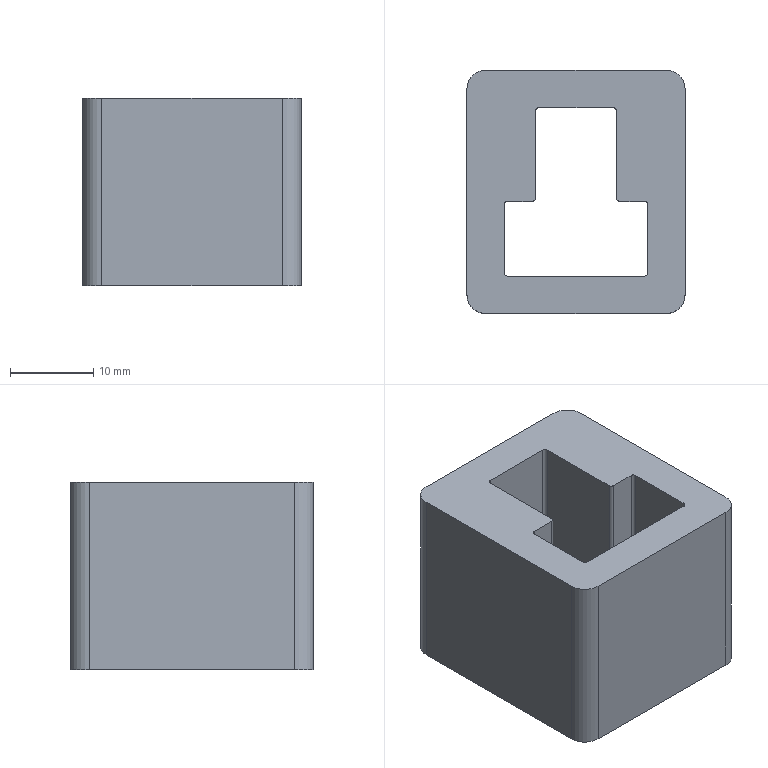Part | Creo | features DATUM PLANE 3, COORDINATE SYSTEM 1, CURVE 1, PROTRUSION 1 | 1 solid | 26 faces | box 26.25 x 29.25 x 22.5 mm | volume 11220 mm3 | plane 14 | cylinder 12 | commonest cylinder face diameters 0.75 x8 4.5 x4
STEP:
#1=CARTESIAN_POINT('',(0.,0.,0.));
#2=DIRECTION('',(0.,0.,1.));
#3=DIRECTION('',(1.,0.,0.));
#4=AXIS2_PLACEMENT_3D('',#1,#2,#3);
#5=CARTESIAN_POINT('',(-10.472,14.408,0.));
#6=VERTEX_POINT('',#5);
#7=CARTESIAN_POINT('',(-10.472,-10.342,0.));
#8=VERTEX_POINT('',#7);
#9=CARTESIAN_POINT('',(-10.472,14.408,0.));
#10=DIRECTION('',(0.,-1.,0.));
#11=VECTOR('',#10,24.75);
#12=LINE('',#9,#11);
#13=EDGE_CURVE('',#6,#8,#12,.T.);
#14=ORIENTED_EDGE('',*,*,#13,.T.);
#15=CARTESIAN_POINT('',(-8.222,-12.592,0.));
#16=VERTEX_POINT('',#15);
#17=CARTESIAN_POINT('',(-8.222,-10.342,0.));
#18=DIRECTION('',(0.,0.,1.));
#19=DIRECTION('',(-1.,0.,0.));
#20=AXIS2_PLACEMENT_3D('',#17,#18,#19);
#21=CIRCLE('',#20,2.25);
#22=EDGE_CURVE('',#8,#16,#21,.T.);
#23=ORIENTED_EDGE('',*,*,#22,.T.);
#24=CARTESIAN_POINT('',(13.528,-12.592,0.));
#25=VERTEX_POINT('',#24);
#26=CARTESIAN_POINT('',(-8.222,-12.592,0.));
#27=DIRECTION('',(1.,0.,0.));
#28=VECTOR('',#27,21.75);
#29=LINE('',#26,#28);
#30=EDGE_CURVE('',#16,#25,#29,.T.);
#31=ORIENTED_EDGE('',*,*,#30,.T.);
#32=CARTESIAN_POINT('',(15.778,-10.342,0.));
#33=VERTEX_POINT('',#32);
#34=CARTESIAN_POINT('',(13.528,-10.342,0.));
#35=DIRECTION('',(0.,0.,1.));
#36=DIRECTION('',(0.,-1.,0.));
#37=AXIS2_PLACEMENT_3D('',#34,#35,#36);
#38=CIRCLE('',#37,2.25);
#39=EDGE_CURVE('',#25,#33,#38,.T.);
#40=ORIENTED_EDGE('',*,*,#39,.T.);
#41=CARTESIAN_POINT('',(15.778,14.408,0.));
#42=VERTEX_POINT('',#41);
#43=CARTESIAN_POINT('',(15.778,-10.342,0.));
#44=DIRECTION('',(0.,1.,0.));
#45=VECTOR('',#44,24.75);
#46=LINE('',#43,#45);
#47=EDGE_CURVE('',#33,#42,#46,.T.);
#48=ORIENTED_EDGE('',*,*,#47,.T.);
#49=CARTESIAN_POINT('',(13.528,16.658,0.));
#50=VERTEX_POINT('',#49);
#51=CARTESIAN_POINT('',(13.528,14.408,0.));
#52=DIRECTION('',(0.,0.,1.));
#53=DIRECTION('',(1.,0.,0.));
#54=AXIS2_PLACEMENT_3D('',#51,#52,#53);
#55=CIRCLE('',#54,2.25);
#56=EDGE_CURVE('',#42,#50,#55,.T.);
#57=ORIENTED_EDGE('',*,*,#56,.T.);
#58=CARTESIAN_POINT('',(-8.222,16.658,0.));
#59=VERTEX_POINT('',#58);
#60=CARTESIAN_POINT('',(13.528,16.658,0.));
#61=DIRECTION('',(-1.,0.,0.));
#62=VECTOR('',#61,21.75);
#63=LINE('',#60,#62);
#64=EDGE_CURVE('',#50,#59,#63,.T.);
#65=ORIENTED_EDGE('',*,*,#64,.T.);
#66=CARTESIAN_POINT('',(-8.222,14.408,0.));
#67=DIRECTION('',(0.,0.,1.));
#68=DIRECTION('',(0.,1.,0.));
#69=AXIS2_PLACEMENT_3D('',#66,#67,#68);
#70=CIRCLE('',#69,2.25);
#71=EDGE_CURVE('',#59,#6,#70,.T.);
#72=ORIENTED_EDGE('',*,*,#71,.T.);
#73=EDGE_LOOP('',(#14,#23,#31,#40,#48,#57,#65,#72));
#74=FACE_OUTER_BOUND('',#73,.F.);
#75=CARTESIAN_POINT('',(-2.222,11.783,0.));
#76=VERTEX_POINT('',#75);
#77=CARTESIAN_POINT('',(-1.847,12.158,0.));
#78=VERTEX_POINT('',#77);
#79=CARTESIAN_POINT('',(-1.847,11.783,0.));
#80=DIRECTION('',(0.,0.,-1.));
#81=DIRECTION('',(-1.,0.,0.));
#82=AXIS2_PLACEMENT_3D('',#79,#80,#81);
#83=CIRCLE('',#82,0.375);
#84=EDGE_CURVE('',#76,#78,#83,.T.);
#85=ORIENTED_EDGE('',*,*,#84,.T.);
#86=CARTESIAN_POINT('',(7.153,12.158,0.));
#87=VERTEX_POINT('',#86);
#88=CARTESIAN_POINT('',(-1.847,12.158,0.));
#89=DIRECTION('',(1.,0.,0.));
#90=VECTOR('',#89,9.);
#91=LINE('',#88,#90);
#92=EDGE_CURVE('',#78,#87,#91,.T.);
#93=ORIENTED_EDGE('',*,*,#92,.T.);
#94=CARTESIAN_POINT('',(7.528,11.783,0.));
#95=VERTEX_POINT('',#94);
#96=CARTESIAN_POINT('',(7.153,11.783,0.));
#97=DIRECTION('',(0.,0.,-1.));
#98=DIRECTION('',(0.,1.,0.));
#99=AXIS2_PLACEMENT_3D('',#96,#97,#98);
#100=CIRCLE('',#99,0.375);
#101=EDGE_CURVE('',#87,#95,#100,.T.);
#102=ORIENTED_EDGE('',*,*,#101,.T.);
#103=CARTESIAN_POINT('',(7.528,1.283,0.));
#104=VERTEX_POINT('',#103);
#105=CARTESIAN_POINT('',(7.528,11.783,0.));
#106=DIRECTION('',(0.,-1.,0.));
#107=VECTOR('',#106,10.5);
#108=LINE('',#105,#107);
#109=EDGE_CURVE('',#95,#104,#108,.T.);
#110=ORIENTED_EDGE('',*,*,#109,.T.);
#111=CARTESIAN_POINT('',(7.903,0.9081,0.));
#112=VERTEX_POINT('',#111);
#113=CARTESIAN_POINT('',(7.903,1.283,0.));
#114=DIRECTION('',(0.,0.,1.));
#115=DIRECTION('',(-1.,0.,0.));
#116=AXIS2_PLACEMENT_3D('',#113,#114,#115);
#117=CIRCLE('',#116,0.375);
#118=EDGE_CURVE('',#104,#112,#117,.T.);
#119=ORIENTED_EDGE('',*,*,#118,.T.);
#120=CARTESIAN_POINT('',(10.903,0.9081,0.));
#121=VERTEX_POINT('',#120);
#122=CARTESIAN_POINT('',(7.903,0.9081,0.));
#123=DIRECTION('',(1.,0.,0.));
#124=VECTOR('',#123,3.);
#125=LINE('',#122,#124);
#126=EDGE_CURVE('',#112,#121,#125,.T.);
#127=ORIENTED_EDGE('',*,*,#126,.T.);
#128=CARTESIAN_POINT('',(11.278,0.5331,0.));
#129=VERTEX_POINT('',#128);
#130=CARTESIAN_POINT('',(10.903,0.5331,0.));
#131=DIRECTION('',(0.,0.,-1.));
#132=DIRECTION('',(0.,1.,0.));
#133=AXIS2_PLACEMENT_3D('',#130,#131,#132);
#134=CIRCLE('',#133,0.375);
#135=EDGE_CURVE('',#121,#129,#134,.T.);
#136=ORIENTED_EDGE('',*,*,#135,.T.);
#137=CARTESIAN_POINT('',(11.278,-7.717,0.));
#138=VERTEX_POINT('',#137);
#139=CARTESIAN_POINT('',(11.278,0.5331,0.));
#140=DIRECTION('',(0.,-1.,0.));
#141=VECTOR('',#140,8.25);
#142=LINE('',#139,#141);
#143=EDGE_CURVE('',#129,#138,#142,.T.);
#144=ORIENTED_EDGE('',*,*,#143,.T.);
#145=CARTESIAN_POINT('',(10.903,-8.092,0.));
#146=VERTEX_POINT('',#145);
#147=CARTESIAN_POINT('',(10.903,-7.717,0.));
#148=DIRECTION('',(0.,0.,-1.));
#149=DIRECTION('',(1.,0.,0.));
#150=AXIS2_PLACEMENT_3D('',#147,#148,#149);
#151=CIRCLE('',#150,0.375);
#152=EDGE_CURVE('',#138,#146,#151,.T.);
#153=ORIENTED_EDGE('',*,*,#152,.T.);
#154=CARTESIAN_POINT('',(-5.597,-8.092,0.));
#155=VERTEX_POINT('',#154);
#156=CARTESIAN_POINT('',(10.903,-8.092,0.));
#157=DIRECTION('',(-1.,0.,0.));
#158=VECTOR('',#157,16.5);
#159=LINE('',#156,#158);
#160=EDGE_CURVE('',#146,#155,#159,.T.);
#161=ORIENTED_EDGE('',*,*,#160,.T.);
#162=CARTESIAN_POINT('',(-5.972,-7.717,0.));
#163=VERTEX_POINT('',#162);
#164=CARTESIAN_POINT('',(-5.597,-7.717,0.));
#165=DIRECTION('',(0.,0.,-1.));
#166=DIRECTION('',(0.,-1.,0.));
#167=AXIS2_PLACEMENT_3D('',#164,#165,#166);
#168=CIRCLE('',#167,0.375);
#169=EDGE_CURVE('',#155,#163,#168,.T.);
#170=ORIENTED_EDGE('',*,*,#169,.T.);
#171=CARTESIAN_POINT('',(-5.972,0.5331,0.));
#172=VERTEX_POINT('',#171);
#173=CARTESIAN_POINT('',(-5.972,-7.717,0.));
#174=DIRECTION('',(0.,1.,0.));
#175=VECTOR('',#174,8.25);
#176=LINE('',#173,#175);
#177=EDGE_CURVE('',#163,#172,#176,.T.);
#178=ORIENTED_EDGE('',*,*,#177,.T.);
#179=CARTESIAN_POINT('',(-5.597,0.9081,0.));
#180=VERTEX_POINT('',#179);
#181=CARTESIAN_POINT('',(-5.597,0.5331,0.));
#182=DIRECTION('',(0.,0.,-1.));
#183=DIRECTION('',(-1.,0.,0.));
#184=AXIS2_PLACEMENT_3D('',#181,#182,#183);
#185=CIRCLE('',#184,0.375);
#186=EDGE_CURVE('',#172,#180,#185,.T.);
#187=ORIENTED_EDGE('',*,*,#186,.T.);
#188=CARTESIAN_POINT('',(-2.597,0.9081,0.));
#189=VERTEX_POINT('',#188);
#190=CARTESIAN_POINT('',(-5.597,0.9081,0.));
#191=DIRECTION('',(1.,0.,0.));
#192=VECTOR('',#191,3.);
#193=LINE('',#190,#192);
#194=EDGE_CURVE('',#180,#189,#193,.T.);
#195=ORIENTED_EDGE('',*,*,#194,.T.);
#196=CARTESIAN_POINT('',(-2.222,1.283,0.));
#197=VERTEX_POINT('',#196);
#198=CARTESIAN_POINT('',(-2.597,1.283,0.));
#199=DIRECTION('',(0.,0.,1.));
#200=DIRECTION('',(0.,-1.,0.));
#201=AXIS2_PLACEMENT_3D('',#198,#199,#200);
#202=CIRCLE('',#201,0.375);
#203=EDGE_CURVE('',#189,#197,#202,.T.);
#204=ORIENTED_EDGE('',*,*,#203,.T.);
#205=CARTESIAN_POINT('',(-2.222,1.283,0.));
#206=DIRECTION('',(0.,1.,0.));
#207=VECTOR('',#206,10.5);
#208=LINE('',#205,#207);
#209=EDGE_CURVE('',#197,#76,#208,.T.);
#210=ORIENTED_EDGE('',*,*,#209,.T.);
#211=EDGE_LOOP('',(#85,#93,#102,#110,#119,#127,#136,#144,#153,#161,#170,#178,#187,#195,#204,#210));
#212=FACE_BOUND('',#211,.F.);
#213=CARTESIAN_POINT('',(0.,0.,0.));
#214=DIRECTION('',(0.,0.,1.));
#215=DIRECTION('',(1.,0.,0.));
#216=AXIS2_PLACEMENT_3D('',#213,#214,#215);
#217=PLANE('',#216);
#218=ADVANCED_FACE('',(#74,#212),#217,.F.);
#219=ORIENTED_EDGE('',*,*,#84,.F.);
#220=CARTESIAN_POINT('',(-2.222,11.783,22.5));
#221=VERTEX_POINT('',#220);
#222=CARTESIAN_POINT('',(-2.222,11.783,0.));
#223=DIRECTION('',(0.,0.,1.));
#224=VECTOR('',#223,22.5);
#225=LINE('',#222,#224);
#226=EDGE_CURVE('',#76,#221,#225,.T.);
#227=ORIENTED_EDGE('',*,*,#226,.T.);
#228=CARTESIAN_POINT('',(-1.847,12.158,22.5));
#229=VERTEX_POINT('',#228);
#230=CARTESIAN_POINT('',(-1.847,11.783,22.5));
#231=DIRECTION('',(0.,0.,-1.));
#232=DIRECTION('',(-1.,0.,0.));
#233=AXIS2_PLACEMENT_3D('',#230,#231,#232);
#234=CIRCLE('',#233,0.375);
#235=EDGE_CURVE('',#221,#229,#234,.T.);
#236=ORIENTED_EDGE('',*,*,#235,.T.);
#237=CARTESIAN_POINT('',(-1.847,12.158,0.));
#238=DIRECTION('',(0.,0.,1.));
#239=VECTOR('',#238,22.5);
#240=LINE('',#237,#239);
#241=EDGE_CURVE('',#78,#229,#240,.T.);
#242=ORIENTED_EDGE('',*,*,#241,.F.);
#243=EDGE_LOOP('',(#219,#227,#236,#242));
#244=FACE_OUTER_BOUND('',#243,.F.);
#245=CARTESIAN_POINT('',(-1.847,11.783,0.));
#246=DIRECTION('',(0.,0.,1.));
#247=DIRECTION('',(1.,0.,0.));
#248=AXIS2_PLACEMENT_3D('',#245,#246,#247);
#249=CYLINDRICAL_SURFACE('',#248,0.375);
#250=ADVANCED_FACE('',(#244),#249,.F.);
#251=ORIENTED_EDGE('',*,*,#209,.F.);
#252=CARTESIAN_POINT('',(-2.222,1.283,22.5));
#253=VERTEX_POINT('',#252);
#254=CARTESIAN_POINT('',(-2.222,1.283,0.));
#255=DIRECTION('',(0.,0.,1.));
#256=VECTOR('',#255,22.5);
#257=LINE('',#254,#256);
#258=EDGE_CURVE('',#197,#253,#257,.T.);
#259=ORIENTED_EDGE('',*,*,#258,.T.);
#260=CARTESIAN_POINT('',(-2.222,1.283,22.5));
#261=DIRECTION('',(0.,1.,0.));
#262=VECTOR('',#261,10.5);
#263=LINE('',#260,#262);
#264=EDGE_CURVE('',#253,#221,#263,.T.);
#265=ORIENTED_EDGE('',*,*,#264,.T.);
#266=ORIENTED_EDGE('',*,*,#226,.F.);
#267=EDGE_LOOP('',(#251,#259,#265,#266));
#268=FACE_OUTER_BOUND('',#267,.F.);
#269=CARTESIAN_POINT('',(-2.222,1.283,0.));
#270=DIRECTION('',(1.,0.,0.));
#271=DIRECTION('',(0.,1.,0.));
#272=AXIS2_PLACEMENT_3D('',#269,#270,#271);
#273=PLANE('',#272);
#274=ADVANCED_FACE('',(#268),#273,.T.);
#275=ORIENTED_EDGE('',*,*,#203,.F.);
#276=CARTESIAN_POINT('',(-2.597,0.9081,22.5));
#277=VERTEX_POINT('',#276);
#278=CARTESIAN_POINT('',(-2.597,0.9081,0.));
#279=DIRECTION('',(0.,0.,1.));
#280=VECTOR('',#279,22.5);
#281=LINE('',#278,#280);
#282=EDGE_CURVE('',#189,#277,#281,.T.);
#283=ORIENTED_EDGE('',*,*,#282,.T.);
#284=CARTESIAN_POINT('',(-2.597,1.283,22.5));
#285=DIRECTION('',(0.,0.,1.));
#286=DIRECTION('',(0.,-1.,0.));
#287=AXIS2_PLACEMENT_3D('',#284,#285,#286);
#288=CIRCLE('',#287,0.375);
#289=EDGE_CURVE('',#277,#253,#288,.T.);
#290=ORIENTED_EDGE('',*,*,#289,.T.);
#291=ORIENTED_EDGE('',*,*,#258,.F.);
#292=EDGE_LOOP('',(#275,#283,#290,#291));
#293=FACE_OUTER_BOUND('',#292,.F.);
#294=CARTESIAN_POINT('',(-2.597,1.283,0.));
#295=DIRECTION('',(0.,0.,1.));
#296=DIRECTION('',(1.,0.,0.));
#297=AXIS2_PLACEMENT_3D('',#294,#295,#296);
#298=CYLINDRICAL_SURFACE('',#297,0.375);
#299=ADVANCED_FACE('',(#293),#298,.T.);
#300=ORIENTED_EDGE('',*,*,#194,.F.);
#301=CARTESIAN_POINT('',(-5.597,0.9081,22.5));
#302=VERTEX_POINT('',#301);
#303=CARTESIAN_POINT('',(-5.597,0.9081,0.));
#304=DIRECTION('',(0.,0.,1.));
#305=VECTOR('',#304,22.5);
#306=LINE('',#303,#305);
#307=EDGE_CURVE('',#180,#302,#306,.T.);
#308=ORIENTED_EDGE('',*,*,#307,.T.);
#309=CARTESIAN_POINT('',(-5.597,0.9081,22.5));
#310=DIRECTION('',(1.,0.,0.));
#311=VECTOR('',#310,3.);
#312=LINE('',#309,#311);
#313=EDGE_CURVE('',#302,#277,#312,.T.);
#314=ORIENTED_EDGE('',*,*,#313,.T.);
#315=ORIENTED_EDGE('',*,*,#282,.F.);
#316=EDGE_LOOP('',(#300,#308,#314,#315));
#317=FACE_OUTER_BOUND('',#316,.F.);
#318=CARTESIAN_POINT('',(-5.597,0.9081,0.));
#319=DIRECTION('',(0.,-1.,0.));
#320=DIRECTION('',(1.,0.,0.));
#321=AXIS2_PLACEMENT_3D('',#318,#319,#320);
#322=PLANE('',#321);
#323=ADVANCED_FACE('',(#317),#322,.T.);
#324=ORIENTED_EDGE('',*,*,#186,.F.);
#325=CARTESIAN_POINT('',(-5.972,0.5331,22.5));
#326=VERTEX_POINT('',#325);
#327=CARTESIAN_POINT('',(-5.972,0.5331,0.));
#328=DIRECTION('',(0.,0.,1.));
#329=VECTOR('',#328,22.5);
#330=LINE('',#327,#329);
#331=EDGE_CURVE('',#172,#326,#330,.T.);
#332=ORIENTED_EDGE('',*,*,#331,.T.);
#333=CARTESIAN_POINT('',(-5.597,0.5331,22.5));
#334=DIRECTION('',(0.,0.,-1.));
#335=DIRECTION('',(-1.,0.,0.));
#336=AXIS2_PLACEMENT_3D('',#333,#334,#335);
#337=CIRCLE('',#336,0.375);
#338=EDGE_CURVE('',#326,#302,#337,.T.);
#339=ORIENTED_EDGE('',*,*,#338,.T.);
#340=ORIENTED_EDGE('',*,*,#307,.F.);
#341=EDGE_LOOP('',(#324,#332,#339,#340));
#342=FACE_OUTER_BOUND('',#341,.F.);
#343=CARTESIAN_POINT('',(-5.597,0.5331,0.));
#344=DIRECTION('',(0.,0.,1.));
#345=DIRECTION('',(1.,0.,0.));
#346=AXIS2_PLACEMENT_3D('',#343,#344,#345);
#347=CYLINDRICAL_SURFACE('',#346,0.375);
#348=ADVANCED_FACE('',(#342),#347,.F.);
#349=ORIENTED_EDGE('',*,*,#177,.F.);
#350=CARTESIAN_POINT('',(-5.972,-7.717,22.5));
#351=VERTEX_POINT('',#350);
#352=CARTESIAN_POINT('',(-5.972,-7.717,0.));
#353=DIRECTION('',(0.,0.,1.));
#354=VECTOR('',#353,22.5);
#355=LINE('',#352,#354);
#356=EDGE_CURVE('',#163,#351,#355,.T.);
#357=ORIENTED_EDGE('',*,*,#356,.T.);
#358=CARTESIAN_POINT('',(-5.972,-7.717,22.5));
#359=DIRECTION('',(0.,1.,0.));
#360=VECTOR('',#359,8.25);
#361=LINE('',#358,#360);
#362=EDGE_CURVE('',#351,#326,#361,.T.);
#363=ORIENTED_EDGE('',*,*,#362,.T.);
#364=ORIENTED_EDGE('',*,*,#331,.F.);
#365=EDGE_LOOP('',(#349,#357,#363,#364));
#366=FACE_OUTER_BOUND('',#365,.F.);
#367=CARTESIAN_POINT('',(-5.972,-7.717,0.));
#368=DIRECTION('',(1.,0.,0.));
#369=DIRECTION('',(0.,1.,0.));
#370=AXIS2_PLACEMENT_3D('',#367,#368,#369);
#371=PLANE('',#370);
#372=ADVANCED_FACE('',(#366),#371,.T.);
#373=ORIENTED_EDGE('',*,*,#169,.F.);
#374=CARTESIAN_POINT('',(-5.597,-8.092,22.5));
#375=VERTEX_POINT('',#374);
#376=CARTESIAN_POINT('',(-5.597,-8.092,0.));
#377=DIRECTION('',(0.,0.,1.));
#378=VECTOR('',#377,22.5);
#379=LINE('',#376,#378);
#380=EDGE_CURVE('',#155,#375,#379,.T.);
#381=ORIENTED_EDGE('',*,*,#380,.T.);
#382=CARTESIAN_POINT('',(-5.597,-7.717,22.5));
#383=DIRECTION('',(0.,0.,-1.));
#384=DIRECTION('',(0.,-1.,0.));
#385=AXIS2_PLACEMENT_3D('',#382,#383,#384);
#386=CIRCLE('',#385,0.375);
#387=EDGE_CURVE('',#375,#351,#386,.T.);
#388=ORIENTED_EDGE('',*,*,#387,.T.);
#389=ORIENTED_EDGE('',*,*,#356,.F.);
#390=EDGE_LOOP('',(#373,#381,#388,#389));
#391=FACE_OUTER_BOUND('',#390,.F.);
#392=CARTESIAN_POINT('',(-5.597,-7.717,0.));
#393=DIRECTION('',(0.,0.,1.));
#394=DIRECTION('',(1.,0.,0.));
#395=AXIS2_PLACEMENT_3D('',#392,#393,#394);
#396=CYLINDRICAL_SURFACE('',#395,0.375);
#397=ADVANCED_FACE('',(#391),#396,.F.);
#398=ORIENTED_EDGE('',*,*,#160,.F.);
#399=CARTESIAN_POINT('',(10.903,-8.092,22.5));
#400=VERTEX_POINT('',#399);
#401=CARTESIAN_POINT('',(10.903,-8.092,0.));
#402=DIRECTION('',(0.,0.,1.));
#403=VECTOR('',#402,22.5);
#404=LINE('',#401,#403);
#405=EDGE_CURVE('',#146,#400,#404,.T.);
#406=ORIENTED_EDGE('',*,*,#405,.T.);
#407=CARTESIAN_POINT('',(10.903,-8.092,22.5));
#408=DIRECTION('',(-1.,0.,0.));
#409=VECTOR('',#408,16.5);
#410=LINE('',#407,#409);
#411=EDGE_CURVE('',#400,#375,#410,.T.);
#412=ORIENTED_EDGE('',*,*,#411,.T.);
#413=ORIENTED_EDGE('',*,*,#380,.F.);
#414=EDGE_LOOP('',(#398,#406,#412,#413));
#415=FACE_OUTER_BOUND('',#414,.F.);
#416=CARTESIAN_POINT('',(10.903,-8.092,0.));
#417=DIRECTION('',(0.,1.,0.));
#418=DIRECTION('',(-1.,0.,0.));
#419=AXIS2_PLACEMENT_3D('',#416,#417,#418);
#420=PLANE('',#419);
#421=ADVANCED_FACE('',(#415),#420,.T.);
#422=ORIENTED_EDGE('',*,*,#152,.F.);
#423=CARTESIAN_POINT('',(11.278,-7.717,22.5));
#424=VERTEX_POINT('',#423);
#425=CARTESIAN_POINT('',(11.278,-7.717,0.));
#426=DIRECTION('',(0.,0.,1.));
#427=VECTOR('',#426,22.5);
#428=LINE('',#425,#427);
#429=EDGE_CURVE('',#138,#424,#428,.T.);
#430=ORIENTED_EDGE('',*,*,#429,.T.);
#431=CARTESIAN_POINT('',(10.903,-7.717,22.5));
#432=DIRECTION('',(0.,0.,-1.));
#433=DIRECTION('',(1.,0.,0.));
#434=AXIS2_PLACEMENT_3D('',#431,#432,#433);
#435=CIRCLE('',#434,0.375);
#436=EDGE_CURVE('',#424,#400,#435,.T.);
#437=ORIENTED_EDGE('',*,*,#436,.T.);
#438=ORIENTED_EDGE('',*,*,#405,.F.);
#439=EDGE_LOOP('',(#422,#430,#437,#438));
#440=FACE_OUTER_BOUND('',#439,.F.);
#441=CARTESIAN_POINT('',(10.903,-7.717,0.));
#442=DIRECTION('',(0.,0.,1.));
#443=DIRECTION('',(1.,0.,0.));
#444=AXIS2_PLACEMENT_3D('',#441,#442,#443);
#445=CYLINDRICAL_SURFACE('',#444,0.375);
#446=ADVANCED_FACE('',(#440),#445,.F.);
#447=ORIENTED_EDGE('',*,*,#143,.F.);
#448=CARTESIAN_POINT('',(11.278,0.5331,22.5));
#449=VERTEX_POINT('',#448);
#450=CARTESIAN_POINT('',(11.278,0.5331,0.));
#451=DIRECTION('',(0.,0.,1.));
#452=VECTOR('',#451,22.5);
#453=LINE('',#450,#452);
#454=EDGE_CURVE('',#129,#449,#453,.T.);
#455=ORIENTED_EDGE('',*,*,#454,.T.);
#456=CARTESIAN_POINT('',(11.278,0.5331,22.5));
#457=DIRECTION('',(0.,-1.,0.));
#458=VECTOR('',#457,8.25);
#459=LINE('',#456,#458);
#460=EDGE_CURVE('',#449,#424,#459,.T.);
#461=ORIENTED_EDGE('',*,*,#460,.T.);
#462=ORIENTED_EDGE('',*,*,#429,.F.);
#463=EDGE_LOOP('',(#447,#455,#461,#462));
#464=FACE_OUTER_BOUND('',#463,.F.);
#465=CARTESIAN_POINT('',(11.278,0.5331,0.));
#466=DIRECTION('',(-1.,0.,0.));
#467=DIRECTION('',(0.,-1.,0.));
#468=AXIS2_PLACEMENT_3D('',#465,#466,#467);
#469=PLANE('',#468);
#470=ADVANCED_FACE('',(#464),#469,.T.);
#471=ORIENTED_EDGE('',*,*,#135,.F.);
#472=CARTESIAN_POINT('',(10.903,0.9081,22.5));
#473=VERTEX_POINT('',#472);
#474=CARTESIAN_POINT('',(10.903,0.9081,0.));
#475=DIRECTION('',(0.,0.,1.));
#476=VECTOR('',#475,22.5);
#477=LINE('',#474,#476);
#478=EDGE_CURVE('',#121,#473,#477,.T.);
#479=ORIENTED_EDGE('',*,*,#478,.T.);
#480=CARTESIAN_POINT('',(10.903,0.5331,22.5));
#481=DIRECTION('',(0.,0.,-1.));
#482=DIRECTION('',(0.,1.,0.));
#483=AXIS2_PLACEMENT_3D('',#480,#481,#482);
#484=CIRCLE('',#483,0.375);
#485=EDGE_CURVE('',#473,#449,#484,.T.);
#486=ORIENTED_EDGE('',*,*,#485,.T.);
#487=ORIENTED_EDGE('',*,*,#454,.F.);
#488=EDGE_LOOP('',(#471,#479,#486,#487));
#489=FACE_OUTER_BOUND('',#488,.F.);
#490=CARTESIAN_POINT('',(10.903,0.5331,0.));
#491=DIRECTION('',(0.,0.,1.));
#492=DIRECTION('',(1.,0.,0.));
#493=AXIS2_PLACEMENT_3D('',#490,#491,#492);
#494=CYLINDRICAL_SURFACE('',#493,0.375);
#495=ADVANCED_FACE('',(#489),#494,.F.);
#496=ORIENTED_EDGE('',*,*,#126,.F.);
#497=CARTESIAN_POINT('',(7.903,0.9081,22.5));
#498=VERTEX_POINT('',#497);
#499=CARTESIAN_POINT('',(7.903,0.9081,0.));
#500=DIRECTION('',(0.,0.,1.));
#501=VECTOR('',#500,22.5);
#502=LINE('',#499,#501);
#503=EDGE_CURVE('',#112,#498,#502,.T.);
#504=ORIENTED_EDGE('',*,*,#503,.T.);
#505=CARTESIAN_POINT('',(7.903,0.9081,22.5));
#506=DIRECTION('',(1.,0.,0.));
#507=VECTOR('',#506,3.);
#508=LINE('',#505,#507);
#509=EDGE_CURVE('',#498,#473,#508,.T.);
#510=ORIENTED_EDGE('',*,*,#509,.T.);
#511=ORIENTED_EDGE('',*,*,#478,.F.);
#512=EDGE_LOOP('',(#496,#504,#510,#511));
#513=FACE_OUTER_BOUND('',#512,.F.);
#514=CARTESIAN_POINT('',(7.903,0.9081,0.));
#515=DIRECTION('',(0.,-1.,0.));
#516=DIRECTION('',(1.,0.,0.));
#517=AXIS2_PLACEMENT_3D('',#514,#515,#516);
#518=PLANE('',#517);
#519=ADVANCED_FACE('',(#513),#518,.T.);
#520=ORIENTED_EDGE('',*,*,#118,.F.);
#521=CARTESIAN_POINT('',(7.528,1.283,22.5));
#522=VERTEX_POINT('',#521);
#523=CARTESIAN_POINT('',(7.528,1.283,0.));
#524=DIRECTION('',(0.,0.,1.));
#525=VECTOR('',#524,22.5);
#526=LINE('',#523,#525);
#527=EDGE_CURVE('',#104,#522,#526,.T.);
#528=ORIENTED_EDGE('',*,*,#527,.T.);
#529=CARTESIAN_POINT('',(7.903,1.283,22.5));
#530=DIRECTION('',(0.,0.,1.));
#531=DIRECTION('',(-1.,0.,0.));
#532=AXIS2_PLACEMENT_3D('',#529,#530,#531);
#533=CIRCLE('',#532,0.375);
#534=EDGE_CURVE('',#522,#498,#533,.T.);
#535=ORIENTED_EDGE('',*,*,#534,.T.);
#536=ORIENTED_EDGE('',*,*,#503,.F.);
#537=EDGE_LOOP('',(#520,#528,#535,#536));
#538=FACE_OUTER_BOUND('',#537,.F.);
#539=CARTESIAN_POINT('',(7.903,1.283,0.));
#540=DIRECTION('',(0.,0.,1.));
#541=DIRECTION('',(1.,0.,0.));
#542=AXIS2_PLACEMENT_3D('',#539,#540,#541);
#543=CYLINDRICAL_SURFACE('',#542,0.375);
#544=ADVANCED_FACE('',(#538),#543,.T.);
#545=ORIENTED_EDGE('',*,*,#109,.F.);
#546=CARTESIAN_POINT('',(7.528,11.783,22.5));
#547=VERTEX_POINT('',#546);
#548=CARTESIAN_POINT('',(7.528,11.783,0.));
#549=DIRECTION('',(0.,0.,1.));
#550=VECTOR('',#549,22.5);
#551=LINE('',#548,#550);
#552=EDGE_CURVE('',#95,#547,#551,.T.);
#553=ORIENTED_EDGE('',*,*,#552,.T.);
#554=CARTESIAN_POINT('',(7.528,11.783,22.5));
#555=DIRECTION('',(0.,-1.,0.));
#556=VECTOR('',#555,10.5);
#557=LINE('',#554,#556);
#558=EDGE_CURVE('',#547,#522,#557,.T.);
#559=ORIENTED_EDGE('',*,*,#558,.T.);
#560=ORIENTED_EDGE('',*,*,#527,.F.);
#561=EDGE_LOOP('',(#545,#553,#559,#560));
#562=FACE_OUTER_BOUND('',#561,.F.);
#563=CARTESIAN_POINT('',(7.528,11.783,0.));
#564=DIRECTION('',(-1.,0.,0.));
#565=DIRECTION('',(0.,-1.,0.));
#566=AXIS2_PLACEMENT_3D('',#563,#564,#565);
#567=PLANE('',#566);
#568=ADVANCED_FACE('',(#562),#567,.T.);
#569=ORIENTED_EDGE('',*,*,#101,.F.);
#570=CARTESIAN_POINT('',(7.153,12.158,22.5));
#571=VERTEX_POINT('',#570);
#572=CARTESIAN_POINT('',(7.153,12.158,0.));
#573=DIRECTION('',(0.,0.,1.));
#574=VECTOR('',#573,22.5);
#575=LINE('',#572,#574);
#576=EDGE_CURVE('',#87,#571,#575,.T.);
#577=ORIENTED_EDGE('',*,*,#576,.T.);
#578=CARTESIAN_POINT('',(7.153,11.783,22.5));
#579=DIRECTION('',(0.,0.,-1.));
#580=DIRECTION('',(0.,1.,0.));
#581=AXIS2_PLACEMENT_3D('',#578,#579,#580);
#582=CIRCLE('',#581,0.375);
#583=EDGE_CURVE('',#571,#547,#582,.T.);
#584=ORIENTED_EDGE('',*,*,#583,.T.);
#585=ORIENTED_EDGE('',*,*,#552,.F.);
#586=EDGE_LOOP('',(#569,#577,#584,#585));
#587=FACE_OUTER_BOUND('',#586,.F.);
#588=CARTESIAN_POINT('',(7.153,11.783,0.));
#589=DIRECTION('',(0.,0.,1.));
#590=DIRECTION('',(1.,0.,0.));
#591=AXIS2_PLACEMENT_3D('',#588,#589,#590);
#592=CYLINDRICAL_SURFACE('',#591,0.375);
#593=ADVANCED_FACE('',(#587),#592,.F.);
#594=ORIENTED_EDGE('',*,*,#92,.F.);
#595=ORIENTED_EDGE('',*,*,#241,.T.);
#596=CARTESIAN_POINT('',(-1.847,12.158,22.5));
#597=DIRECTION('',(1.,0.,0.));
#598=VECTOR('',#597,9.);
#599=LINE('',#596,#598);
#600=EDGE_CURVE('',#229,#571,#599,.T.);
#601=ORIENTED_EDGE('',*,*,#600,.T.);
#602=ORIENTED_EDGE('',*,*,#576,.F.);
#603=EDGE_LOOP('',(#594,#595,#601,#602));
#604=FACE_OUTER_BOUND('',#603,.F.);
#605=CARTESIAN_POINT('',(-1.847,12.158,0.));
#606=DIRECTION('',(0.,-1.,0.));
#607=DIRECTION('',(1.,0.,0.));
#608=AXIS2_PLACEMENT_3D('',#605,#606,#607);
#609=PLANE('',#608);
#610=ADVANCED_FACE('',(#604),#609,.T.);
#611=CARTESIAN_POINT('',(-10.472,14.408,22.5));
#612=VERTEX_POINT('',#611);
#613=CARTESIAN_POINT('',(-10.472,-10.342,22.5));
#614=VERTEX_POINT('',#613);
#615=CARTESIAN_POINT('',(-10.472,14.408,22.5));
#616=DIRECTION('',(0.,-1.,0.));
#617=VECTOR('',#616,24.75);
#618=LINE('',#615,#617);
#619=EDGE_CURVE('',#612,#614,#618,.T.);
#620=ORIENTED_EDGE('',*,*,#619,.F.);
#621=CARTESIAN_POINT('',(-8.222,16.658,22.5));
#622=VERTEX_POINT('',#621);
#623=CARTESIAN_POINT('',(-8.222,14.408,22.5));
#624=DIRECTION('',(0.,0.,1.));
#625=DIRECTION('',(0.,1.,0.));
#626=AXIS2_PLACEMENT_3D('',#623,#624,#625);
#627=CIRCLE('',#626,2.25);
#628=EDGE_CURVE('',#622,#612,#627,.T.);
#629=ORIENTED_EDGE('',*,*,#628,.F.);
#630=CARTESIAN_POINT('',(13.528,16.658,22.5));
#631=VERTEX_POINT('',#630);
#632=CARTESIAN_POINT('',(13.528,16.658,22.5));
#633=DIRECTION('',(-1.,0.,0.));
#634=VECTOR('',#633,21.75);
#635=LINE('',#632,#634);
#636=EDGE_CURVE('',#631,#622,#635,.T.);
#637=ORIENTED_EDGE('',*,*,#636,.F.);
#638=CARTESIAN_POINT('',(15.778,14.408,22.5));
#639=VERTEX_POINT('',#638);
#640=CARTESIAN_POINT('',(13.528,14.408,22.5));
#641=DIRECTION('',(0.,0.,1.));
#642=DIRECTION('',(1.,0.,0.));
#643=AXIS2_PLACEMENT_3D('',#640,#641,#642);
#644=CIRCLE('',#643,2.25);
#645=EDGE_CURVE('',#639,#631,#644,.T.);
#646=ORIENTED_EDGE('',*,*,#645,.F.);
#647=CARTESIAN_POINT('',(15.778,-10.342,22.5));
#648=VERTEX_POINT('',#647);
#649=CARTESIAN_POINT('',(15.778,-10.342,22.5));
#650=DIRECTION('',(0.,1.,0.));
#651=VECTOR('',#650,24.75);
#652=LINE('',#649,#651);
#653=EDGE_CURVE('',#648,#639,#652,.T.);
#654=ORIENTED_EDGE('',*,*,#653,.F.);
#655=CARTESIAN_POINT('',(13.528,-12.592,22.5));
#656=VERTEX_POINT('',#655);
#657=CARTESIAN_POINT('',(13.528,-10.342,22.5));
#658=DIRECTION('',(0.,0.,1.));
#659=DIRECTION('',(0.,-1.,0.));
#660=AXIS2_PLACEMENT_3D('',#657,#658,#659);
#661=CIRCLE('',#660,2.25);
#662=EDGE_CURVE('',#656,#648,#661,.T.);
#663=ORIENTED_EDGE('',*,*,#662,.F.);
#664=CARTESIAN_POINT('',(-8.222,-12.592,22.5));
#665=VERTEX_POINT('',#664);
#666=CARTESIAN_POINT('',(-8.222,-12.592,22.5));
#667=DIRECTION('',(1.,0.,0.));
#668=VECTOR('',#667,21.75);
#669=LINE('',#666,#668);
#670=EDGE_CURVE('',#665,#656,#669,.T.);
#671=ORIENTED_EDGE('',*,*,#670,.F.);
#672=CARTESIAN_POINT('',(-8.222,-10.342,22.5));
#673=DIRECTION('',(0.,0.,1.));
#674=DIRECTION('',(-1.,0.,0.));
#675=AXIS2_PLACEMENT_3D('',#672,#673,#674);
#676=CIRCLE('',#675,2.25);
#677=EDGE_CURVE('',#614,#665,#676,.T.);
#678=ORIENTED_EDGE('',*,*,#677,.F.);
#679=EDGE_LOOP('',(#620,#629,#637,#646,#654,#663,#671,#678));
#680=FACE_OUTER_BOUND('',#679,.F.);
#681=ORIENTED_EDGE('',*,*,#235,.F.);
#682=ORIENTED_EDGE('',*,*,#264,.F.);
#683=ORIENTED_EDGE('',*,*,#289,.F.);
#684=ORIENTED_EDGE('',*,*,#313,.F.);
#685=ORIENTED_EDGE('',*,*,#338,.F.);
#686=ORIENTED_EDGE('',*,*,#362,.F.);
#687=ORIENTED_EDGE('',*,*,#387,.F.);
#688=ORIENTED_EDGE('',*,*,#411,.F.);
#689=ORIENTED_EDGE('',*,*,#436,.F.);
#690=ORIENTED_EDGE('',*,*,#460,.F.);
#691=ORIENTED_EDGE('',*,*,#485,.F.);
#692=ORIENTED_EDGE('',*,*,#509,.F.);
#693=ORIENTED_EDGE('',*,*,#534,.F.);
#694=ORIENTED_EDGE('',*,*,#558,.F.);
#695=ORIENTED_EDGE('',*,*,#583,.F.);
#696=ORIENTED_EDGE('',*,*,#600,.F.);
#697=EDGE_LOOP('',(#681,#682,#683,#684,#685,#686,#687,#688,#689,#690,#691,#692,#693,#694,#695,#696));
#698=FACE_BOUND('',#697,.F.);
#699=CARTESIAN_POINT('',(0.,0.,22.5));
#700=DIRECTION('',(0.,0.,1.));
#701=DIRECTION('',(1.,0.,0.));
#702=AXIS2_PLACEMENT_3D('',#699,#700,#701);
#703=PLANE('',#702);
#704=ADVANCED_FACE('',(#680,#698),#703,.T.);
#705=ORIENTED_EDGE('',*,*,#13,.F.);
#706=CARTESIAN_POINT('',(-10.472,14.408,0.));
#707=DIRECTION('',(0.,0.,1.));
#708=VECTOR('',#707,22.5);
#709=LINE('',#706,#708);
#710=EDGE_CURVE('',#6,#612,#709,.T.);
#711=ORIENTED_EDGE('',*,*,#710,.T.);
#712=ORIENTED_EDGE('',*,*,#619,.T.);
#713=CARTESIAN_POINT('',(-10.472,-10.342,0.));
#714=DIRECTION('',(0.,0.,1.));
#715=VECTOR('',#714,22.5);
#716=LINE('',#713,#715);
#717=EDGE_CURVE('',#8,#614,#716,.T.);
#718=ORIENTED_EDGE('',*,*,#717,.F.);
#719=EDGE_LOOP('',(#705,#711,#712,#718));
#720=FACE_OUTER_BOUND('',#719,.F.);
#721=CARTESIAN_POINT('',(-10.472,14.408,0.));
#722=DIRECTION('',(-1.,0.,0.));
#723=DIRECTION('',(0.,-1.,0.));
#724=AXIS2_PLACEMENT_3D('',#721,#722,#723);
#725=PLANE('',#724);
#726=ADVANCED_FACE('',(#720),#725,.T.);
#727=ORIENTED_EDGE('',*,*,#71,.F.);
#728=CARTESIAN_POINT('',(-8.222,16.658,0.));
#729=DIRECTION('',(0.,0.,1.));
#730=VECTOR('',#729,22.5);
#731=LINE('',#728,#730);
#732=EDGE_CURVE('',#59,#622,#731,.T.);
#733=ORIENTED_EDGE('',*,*,#732,.T.);
#734=ORIENTED_EDGE('',*,*,#628,.T.);
#735=ORIENTED_EDGE('',*,*,#710,.F.);
#736=EDGE_LOOP('',(#727,#733,#734,#735));
#737=FACE_OUTER_BOUND('',#736,.F.);
#738=CARTESIAN_POINT('',(-8.222,14.408,0.));
#739=DIRECTION('',(0.,0.,1.));
#740=DIRECTION('',(1.,0.,0.));
#741=AXIS2_PLACEMENT_3D('',#738,#739,#740);
#742=CYLINDRICAL_SURFACE('',#741,2.25);
#743=ADVANCED_FACE('',(#737),#742,.T.);
#744=ORIENTED_EDGE('',*,*,#64,.F.);
#745=CARTESIAN_POINT('',(13.528,16.658,0.));
#746=DIRECTION('',(0.,0.,1.));
#747=VECTOR('',#746,22.5);
#748=LINE('',#745,#747);
#749=EDGE_CURVE('',#50,#631,#748,.T.);
#750=ORIENTED_EDGE('',*,*,#749,.T.);
#751=ORIENTED_EDGE('',*,*,#636,.T.);
#752=ORIENTED_EDGE('',*,*,#732,.F.);
#753=EDGE_LOOP('',(#744,#750,#751,#752));
#754=FACE_OUTER_BOUND('',#753,.F.);
#755=CARTESIAN_POINT('',(13.528,16.658,0.));
#756=DIRECTION('',(0.,1.,0.));
#757=DIRECTION('',(-1.,0.,0.));
#758=AXIS2_PLACEMENT_3D('',#755,#756,#757);
#759=PLANE('',#758);
#760=ADVANCED_FACE('',(#754),#759,.T.);
#761=ORIENTED_EDGE('',*,*,#56,.F.);
#762=CARTESIAN_POINT('',(15.778,14.408,0.));
#763=DIRECTION('',(0.,0.,1.));
#764=VECTOR('',#763,22.5);
#765=LINE('',#762,#764);
#766=EDGE_CURVE('',#42,#639,#765,.T.);
#767=ORIENTED_EDGE('',*,*,#766,.T.);
#768=ORIENTED_EDGE('',*,*,#645,.T.);
#769=ORIENTED_EDGE('',*,*,#749,.F.);
#770=EDGE_LOOP('',(#761,#767,#768,#769));
#771=FACE_OUTER_BOUND('',#770,.F.);
#772=CARTESIAN_POINT('',(13.528,14.408,0.));
#773=DIRECTION('',(0.,0.,1.));
#774=DIRECTION('',(1.,0.,0.));
#775=AXIS2_PLACEMENT_3D('',#772,#773,#774);
#776=CYLINDRICAL_SURFACE('',#775,2.25);
#777=ADVANCED_FACE('',(#771),#776,.T.);
#778=ORIENTED_EDGE('',*,*,#47,.F.);
#779=CARTESIAN_POINT('',(15.778,-10.342,0.));
#780=DIRECTION('',(0.,0.,1.));
#781=VECTOR('',#780,22.5);
#782=LINE('',#779,#781);
#783=EDGE_CURVE('',#33,#648,#782,.T.);
#784=ORIENTED_EDGE('',*,*,#783,.T.);
#785=ORIENTED_EDGE('',*,*,#653,.T.);
#786=ORIENTED_EDGE('',*,*,#766,.F.);
#787=EDGE_LOOP('',(#778,#784,#785,#786));
#788=FACE_OUTER_BOUND('',#787,.F.);
#789=CARTESIAN_POINT('',(15.778,-10.342,0.));
#790=DIRECTION('',(1.,0.,0.));
#791=DIRECTION('',(0.,1.,0.));
#792=AXIS2_PLACEMENT_3D('',#789,#790,#791);
#793=PLANE('',#792);
#794=ADVANCED_FACE('',(#788),#793,.T.);
#795=ORIENTED_EDGE('',*,*,#39,.F.);
#796=CARTESIAN_POINT('',(13.528,-12.592,0.));
#797=DIRECTION('',(0.,0.,1.));
#798=VECTOR('',#797,22.5);
#799=LINE('',#796,#798);
#800=EDGE_CURVE('',#25,#656,#799,.T.);
#801=ORIENTED_EDGE('',*,*,#800,.T.);
#802=ORIENTED_EDGE('',*,*,#662,.T.);
#803=ORIENTED_EDGE('',*,*,#783,.F.);
#804=EDGE_LOOP('',(#795,#801,#802,#803));
#805=FACE_OUTER_BOUND('',#804,.F.);
#806=CARTESIAN_POINT('',(13.528,-10.342,0.));
#807=DIRECTION('',(0.,0.,1.));
#808=DIRECTION('',(1.,0.,0.));
#809=AXIS2_PLACEMENT_3D('',#806,#807,#808);
#810=CYLINDRICAL_SURFACE('',#809,2.25);
#811=ADVANCED_FACE('',(#805),#810,.T.);
#812=ORIENTED_EDGE('',*,*,#30,.F.);
#813=CARTESIAN_POINT('',(-8.222,-12.592,0.));
#814=DIRECTION('',(0.,0.,1.));
#815=VECTOR('',#814,22.5);
#816=LINE('',#813,#815);
#817=EDGE_CURVE('',#16,#665,#816,.T.);
#818=ORIENTED_EDGE('',*,*,#817,.T.);
#819=ORIENTED_EDGE('',*,*,#670,.T.);
#820=ORIENTED_EDGE('',*,*,#800,.F.);
#821=EDGE_LOOP('',(#812,#818,#819,#820));
#822=FACE_OUTER_BOUND('',#821,.F.);
#823=CARTESIAN_POINT('',(-8.222,-12.592,0.));
#824=DIRECTION('',(0.,-1.,0.));
#825=DIRECTION('',(1.,0.,0.));
#826=AXIS2_PLACEMENT_3D('',#823,#824,#825);
#827=PLANE('',#826);
#828=ADVANCED_FACE('',(#822),#827,.T.);
#829=ORIENTED_EDGE('',*,*,#22,.F.);
#830=ORIENTED_EDGE('',*,*,#717,.T.);
#831=ORIENTED_EDGE('',*,*,#677,.T.);
#832=ORIENTED_EDGE('',*,*,#817,.F.);
#833=EDGE_LOOP('',(#829,#830,#831,#832));
#834=FACE_OUTER_BOUND('',#833,.F.);
#835=CARTESIAN_POINT('',(-8.222,-10.342,0.));
#836=DIRECTION('',(0.,0.,1.));
#837=DIRECTION('',(1.,0.,0.));
#838=AXIS2_PLACEMENT_3D('',#835,#836,#837);
#839=CYLINDRICAL_SURFACE('',#838,2.25);
#840=ADVANCED_FACE('',(#834),#839,.T.);
#841=CLOSED_SHELL('',(#218,#250,#274,#299,#323,#348,#372,#397,#421,#446,#470,#495,#519,#544,#568,#593,#610,#704,#726,#743,#760,#777,#794,#811,#828,#840));
#842=MANIFOLD_SOLID_BREP('',#841);
#843=(LENGTH_UNIT()NAMED_UNIT(*)SI_UNIT(.MILLI.,.METRE.));
#844=UNCERTAINTY_MEASURE_WITH_UNIT(LENGTH_MEASURE(0.004528),#843,'','');
#845=(NAMED_UNIT(*)PLANE_ANGLE_UNIT()SI_UNIT($,.RADIAN.));
#846=PLANE_ANGLE_MEASURE_WITH_UNIT(PLANE_ANGLE_MEASURE(0.01745),#845);
#847=(CONVERSION_BASED_UNIT('DEGREE',#846)NAMED_UNIT(*)PLANE_ANGLE_UNIT());
#848=(NAMED_UNIT(*)SI_UNIT($,.STERADIAN.)SOLID_ANGLE_UNIT());
#849=(GEOMETRIC_REPRESENTATION_CONTEXT(3)GLOBAL_UNCERTAINTY_ASSIGNED_CONTEXT((#844))GLOBAL_UNIT_ASSIGNED_CONTEXT((#843,#847,#848))REPRESENTATION_CONTEXT('',''));
#850=ADVANCED_BREP_SHAPE_REPRESENTATION('',(#4,#842),#849);